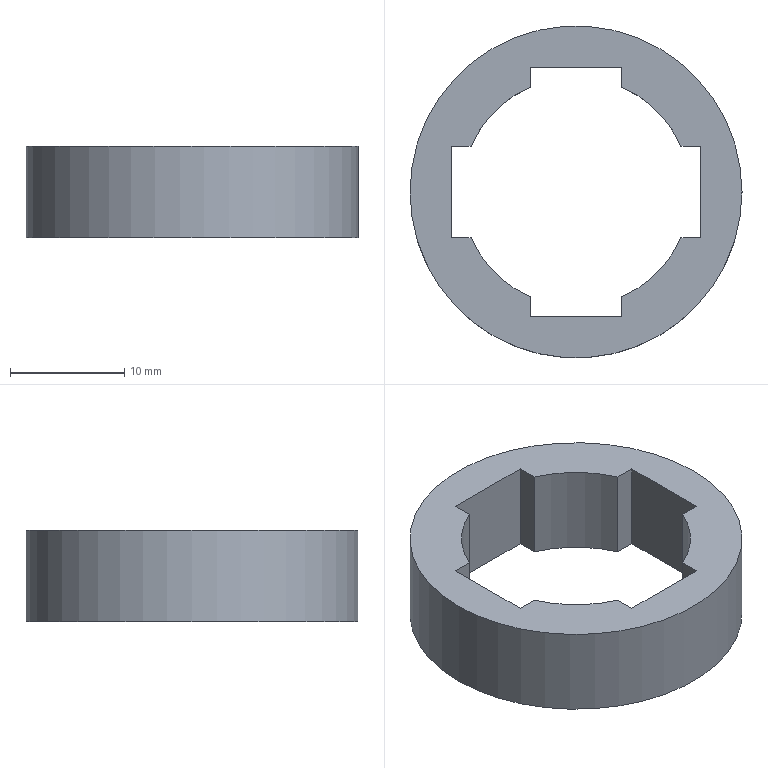Part | NX | features DATUM_CSYS 2, EXTRUDE 1, SKETCH 1 | 1 solid | 19 faces | box 29 x 29 x 8 mm | volume 2471 mm3 | plane 14 | cylinder 5 | commonest cylinder face diameters 20 x4 29 x1
STEP:
#1=CARTESIAN_POINT('',(-10.9,-4.,0.));
#2=VERTEX_POINT('',#1);
#3=CARTESIAN_POINT('',(-10.9,4.,0.));
#4=VERTEX_POINT('',#3);
#5=CARTESIAN_POINT('',(-10.9,2.1,0.));
#6=DIRECTION('',(0.,1.,0.));
#7=VECTOR('',#6,1000.);
#8=LINE('',#5,#7);
#9=EDGE_CURVE('',#2,#4,#8,.T.);
#10=ORIENTED_EDGE('',*,*,#9,.T.);
#11=CARTESIAN_POINT('',(-10.9,4.,8.));
#12=VERTEX_POINT('',#11);
#13=CARTESIAN_POINT('',(-10.9,4.,8.));
#14=DIRECTION('',(0.,0.,-1.));
#15=VECTOR('',#14,1000.);
#16=LINE('',#13,#15);
#17=EDGE_CURVE('',#12,#4,#16,.T.);
#18=ORIENTED_EDGE('',*,*,#17,.F.);
#19=CARTESIAN_POINT('',(-10.9,-4.,8.));
#20=VERTEX_POINT('',#19);
#21=CARTESIAN_POINT('',(-10.9,-4.,8.));
#22=DIRECTION('',(0.,1.,0.));
#23=VECTOR('',#22,1000.);
#24=LINE('',#21,#23);
#25=EDGE_CURVE('',#20,#12,#24,.T.);
#26=ORIENTED_EDGE('',*,*,#25,.F.);
#27=CARTESIAN_POINT('',(-10.9,-4.,8.));
#28=DIRECTION('',(0.,0.,-1.));
#29=VECTOR('',#28,1000.);
#30=LINE('',#27,#29);
#31=EDGE_CURVE('',#20,#2,#30,.T.);
#32=ORIENTED_EDGE('',*,*,#31,.T.);
#33=EDGE_LOOP('',(#10,#18,#26,#32));
#34=FACE_BOUND('',#33,.T.);
#35=CARTESIAN_POINT('',(-10.9,2.1,8.));
#36=DIRECTION('',(-1.,0.,0.));
#37=DIRECTION('',(0.,0.,1.));
#38=AXIS2_PLACEMENT_3D('',#35,#36,#37);
#39=PLANE('',#38);
#40=ADVANCED_FACE('',(#34),#39,.F.);
#41=CARTESIAN_POINT('',(-9.165,4.,0.));
#42=VERTEX_POINT('',#41);
#43=CARTESIAN_POINT('',(-10.9,4.,0.));
#44=DIRECTION('',(1.,0.,0.));
#45=VECTOR('',#44,1000.);
#46=LINE('',#43,#45);
#47=EDGE_CURVE('',#4,#42,#46,.T.);
#48=ORIENTED_EDGE('',*,*,#47,.T.);
#49=CARTESIAN_POINT('',(-9.165,4.,8.));
#50=VERTEX_POINT('',#49);
#51=CARTESIAN_POINT('',(-9.165,4.,8.));
#52=DIRECTION('',(0.,0.,-1.));
#53=VECTOR('',#52,1000.);
#54=LINE('',#51,#53);
#55=EDGE_CURVE('',#50,#42,#54,.T.);
#56=ORIENTED_EDGE('',*,*,#55,.F.);
#57=CARTESIAN_POINT('',(-10.9,4.,8.));
#58=DIRECTION('',(1.,0.,0.));
#59=VECTOR('',#58,1000.);
#60=LINE('',#57,#59);
#61=EDGE_CURVE('',#12,#50,#60,.T.);
#62=ORIENTED_EDGE('',*,*,#61,.F.);
#63=ORIENTED_EDGE('',*,*,#17,.T.);
#64=EDGE_LOOP('',(#48,#56,#62,#63));
#65=FACE_BOUND('',#64,.T.);
#66=CARTESIAN_POINT('',(-10.9,4.,8.));
#67=DIRECTION('',(0.,1.,0.));
#68=DIRECTION('',(0.,0.,1.));
#69=AXIS2_PLACEMENT_3D('',#66,#67,#68);
#70=PLANE('',#69);
#71=ADVANCED_FACE('',(#65),#70,.F.);
#72=CARTESIAN_POINT('',(-4.,9.165,0.));
#73=VERTEX_POINT('',#72);
#74=CARTESIAN_POINT('',(0.,0.,0.));
#75=DIRECTION('',(0.,0.,-1.));
#76=DIRECTION('',(1.,0.,0.));
#77=AXIS2_PLACEMENT_3D('',#74,#75,#76);
#78=CIRCLE('',#77,10.);
#79=EDGE_CURVE('',#42,#73,#78,.T.);
#80=ORIENTED_EDGE('',*,*,#79,.T.);
#81=CARTESIAN_POINT('',(-4.,9.165,8.));
#82=VERTEX_POINT('',#81);
#83=CARTESIAN_POINT('',(-4.,9.165,8.));
#84=DIRECTION('',(0.,0.,-1.));
#85=VECTOR('',#84,1000.);
#86=LINE('',#83,#85);
#87=EDGE_CURVE('',#82,#73,#86,.T.);
#88=ORIENTED_EDGE('',*,*,#87,.F.);
#89=CARTESIAN_POINT('',(0.,0.,8.));
#90=DIRECTION('',(0.,0.,-1.));
#91=DIRECTION('',(1.,0.,0.));
#92=AXIS2_PLACEMENT_3D('',#89,#90,#91);
#93=CIRCLE('',#92,10.);
#94=EDGE_CURVE('',#50,#82,#93,.T.);
#95=ORIENTED_EDGE('',*,*,#94,.F.);
#96=ORIENTED_EDGE('',*,*,#55,.T.);
#97=EDGE_LOOP('',(#80,#88,#95,#96));
#98=FACE_BOUND('',#97,.T.);
#99=CARTESIAN_POINT('',(0.,0.,8.));
#100=DIRECTION('',(0.,0.,-1.));
#101=DIRECTION('',(-1.,0.,0.));
#102=AXIS2_PLACEMENT_3D('',#99,#100,#101);
#103=CYLINDRICAL_SURFACE('',#102,10.);
#104=ADVANCED_FACE('',(#98),#103,.F.);
#105=CARTESIAN_POINT('',(-4.,10.9,0.));
#106=VERTEX_POINT('',#105);
#107=CARTESIAN_POINT('',(-4.,9.165,0.));
#108=DIRECTION('',(0.,1.,0.));
#109=VECTOR('',#108,1000.);
#110=LINE('',#107,#109);
#111=EDGE_CURVE('',#73,#106,#110,.T.);
#112=ORIENTED_EDGE('',*,*,#111,.T.);
#113=CARTESIAN_POINT('',(-4.,10.9,8.));
#114=VERTEX_POINT('',#113);
#115=CARTESIAN_POINT('',(-4.,10.9,8.));
#116=DIRECTION('',(0.,0.,-1.));
#117=VECTOR('',#116,1000.);
#118=LINE('',#115,#117);
#119=EDGE_CURVE('',#114,#106,#118,.T.);
#120=ORIENTED_EDGE('',*,*,#119,.F.);
#121=CARTESIAN_POINT('',(-4.,9.165,8.));
#122=DIRECTION('',(0.,1.,0.));
#123=VECTOR('',#122,1000.);
#124=LINE('',#121,#123);
#125=EDGE_CURVE('',#82,#114,#124,.T.);
#126=ORIENTED_EDGE('',*,*,#125,.F.);
#127=ORIENTED_EDGE('',*,*,#87,.T.);
#128=EDGE_LOOP('',(#112,#120,#126,#127));
#129=FACE_BOUND('',#128,.T.);
#130=CARTESIAN_POINT('',(-4.,9.165,8.));
#131=DIRECTION('',(-1.,0.,0.));
#132=DIRECTION('',(0.,0.,1.));
#133=AXIS2_PLACEMENT_3D('',#130,#131,#132);
#134=PLANE('',#133);
#135=ADVANCED_FACE('',(#129),#134,.F.);
#136=CARTESIAN_POINT('',(4.,10.9,0.));
#137=VERTEX_POINT('',#136);
#138=CARTESIAN_POINT('',(-2.1,10.9,0.));
#139=DIRECTION('',(1.,0.,0.));
#140=VECTOR('',#139,1000.);
#141=LINE('',#138,#140);
#142=EDGE_CURVE('',#106,#137,#141,.T.);
#143=ORIENTED_EDGE('',*,*,#142,.T.);
#144=CARTESIAN_POINT('',(4.,10.9,8.));
#145=VERTEX_POINT('',#144);
#146=CARTESIAN_POINT('',(4.,10.9,8.));
#147=DIRECTION('',(0.,0.,-1.));
#148=VECTOR('',#147,1000.);
#149=LINE('',#146,#148);
#150=EDGE_CURVE('',#145,#137,#149,.T.);
#151=ORIENTED_EDGE('',*,*,#150,.F.);
#152=CARTESIAN_POINT('',(-4.,10.9,8.));
#153=DIRECTION('',(1.,0.,0.));
#154=VECTOR('',#153,1000.);
#155=LINE('',#152,#154);
#156=EDGE_CURVE('',#114,#145,#155,.T.);
#157=ORIENTED_EDGE('',*,*,#156,.F.);
#158=ORIENTED_EDGE('',*,*,#119,.T.);
#159=EDGE_LOOP('',(#143,#151,#157,#158));
#160=FACE_BOUND('',#159,.T.);
#161=CARTESIAN_POINT('',(-2.1,10.9,8.));
#162=DIRECTION('',(0.,1.,0.));
#163=DIRECTION('',(0.,0.,1.));
#164=AXIS2_PLACEMENT_3D('',#161,#162,#163);
#165=PLANE('',#164);
#166=ADVANCED_FACE('',(#160),#165,.F.);
#167=CARTESIAN_POINT('',(4.,9.165,0.));
#168=VERTEX_POINT('',#167);
#169=CARTESIAN_POINT('',(4.,10.9,0.));
#170=DIRECTION('',(0.,-1.,0.));
#171=VECTOR('',#170,1000.);
#172=LINE('',#169,#171);
#173=EDGE_CURVE('',#137,#168,#172,.T.);
#174=ORIENTED_EDGE('',*,*,#173,.T.);
#175=CARTESIAN_POINT('',(4.,9.165,8.));
#176=VERTEX_POINT('',#175);
#177=CARTESIAN_POINT('',(4.,9.165,8.));
#178=DIRECTION('',(0.,0.,-1.));
#179=VECTOR('',#178,1000.);
#180=LINE('',#177,#179);
#181=EDGE_CURVE('',#176,#168,#180,.T.);
#182=ORIENTED_EDGE('',*,*,#181,.F.);
#183=CARTESIAN_POINT('',(4.,10.9,8.));
#184=DIRECTION('',(0.,-1.,0.));
#185=VECTOR('',#184,1000.);
#186=LINE('',#183,#185);
#187=EDGE_CURVE('',#145,#176,#186,.T.);
#188=ORIENTED_EDGE('',*,*,#187,.F.);
#189=ORIENTED_EDGE('',*,*,#150,.T.);
#190=EDGE_LOOP('',(#174,#182,#188,#189));
#191=FACE_BOUND('',#190,.T.);
#192=CARTESIAN_POINT('',(4.,10.9,8.));
#193=DIRECTION('',(1.,0.,0.));
#194=DIRECTION('',(0.,0.,-1.));
#195=AXIS2_PLACEMENT_3D('',#192,#193,#194);
#196=PLANE('',#195);
#197=ADVANCED_FACE('',(#191),#196,.F.);
#198=CARTESIAN_POINT('',(9.165,4.,0.));
#199=VERTEX_POINT('',#198);
#200=CARTESIAN_POINT('',(0.,0.,0.));
#201=DIRECTION('',(0.,0.,-1.));
#202=DIRECTION('',(1.,0.,0.));
#203=AXIS2_PLACEMENT_3D('',#200,#201,#202);
#204=CIRCLE('',#203,10.);
#205=EDGE_CURVE('',#168,#199,#204,.T.);
#206=ORIENTED_EDGE('',*,*,#205,.T.);
#207=CARTESIAN_POINT('',(9.165,4.,8.));
#208=VERTEX_POINT('',#207);
#209=CARTESIAN_POINT('',(9.165,4.,8.));
#210=DIRECTION('',(0.,0.,-1.));
#211=VECTOR('',#210,1000.);
#212=LINE('',#209,#211);
#213=EDGE_CURVE('',#208,#199,#212,.T.);
#214=ORIENTED_EDGE('',*,*,#213,.F.);
#215=CARTESIAN_POINT('',(0.,0.,8.));
#216=DIRECTION('',(0.,0.,-1.));
#217=DIRECTION('',(1.,0.,0.));
#218=AXIS2_PLACEMENT_3D('',#215,#216,#217);
#219=CIRCLE('',#218,10.);
#220=EDGE_CURVE('',#176,#208,#219,.T.);
#221=ORIENTED_EDGE('',*,*,#220,.F.);
#222=ORIENTED_EDGE('',*,*,#181,.T.);
#223=EDGE_LOOP('',(#206,#214,#221,#222));
#224=FACE_BOUND('',#223,.T.);
#225=CARTESIAN_POINT('',(0.,0.,8.));
#226=DIRECTION('',(0.,0.,-1.));
#227=DIRECTION('',(-1.,0.,0.));
#228=AXIS2_PLACEMENT_3D('',#225,#226,#227);
#229=CYLINDRICAL_SURFACE('',#228,10.);
#230=ADVANCED_FACE('',(#224),#229,.F.);
#231=CARTESIAN_POINT('',(10.9,4.,0.));
#232=VERTEX_POINT('',#231);
#233=CARTESIAN_POINT('',(9.165,4.,0.));
#234=DIRECTION('',(1.,0.,0.));
#235=VECTOR('',#234,1000.);
#236=LINE('',#233,#235);
#237=EDGE_CURVE('',#199,#232,#236,.T.);
#238=ORIENTED_EDGE('',*,*,#237,.T.);
#239=CARTESIAN_POINT('',(10.9,4.,8.));
#240=VERTEX_POINT('',#239);
#241=CARTESIAN_POINT('',(10.9,4.,8.));
#242=DIRECTION('',(0.,0.,-1.));
#243=VECTOR('',#242,1000.);
#244=LINE('',#241,#243);
#245=EDGE_CURVE('',#240,#232,#244,.T.);
#246=ORIENTED_EDGE('',*,*,#245,.F.);
#247=CARTESIAN_POINT('',(9.165,4.,8.));
#248=DIRECTION('',(1.,0.,0.));
#249=VECTOR('',#248,1000.);
#250=LINE('',#247,#249);
#251=EDGE_CURVE('',#208,#240,#250,.T.);
#252=ORIENTED_EDGE('',*,*,#251,.F.);
#253=ORIENTED_EDGE('',*,*,#213,.T.);
#254=EDGE_LOOP('',(#238,#246,#252,#253));
#255=FACE_BOUND('',#254,.T.);
#256=CARTESIAN_POINT('',(9.165,4.,8.));
#257=DIRECTION('',(0.,1.,0.));
#258=DIRECTION('',(0.,0.,1.));
#259=AXIS2_PLACEMENT_3D('',#256,#257,#258);
#260=PLANE('',#259);
#261=ADVANCED_FACE('',(#255),#260,.F.);
#262=CARTESIAN_POINT('',(10.9,-4.,0.));
#263=VERTEX_POINT('',#262);
#264=CARTESIAN_POINT('',(10.9,-2.1,0.));
#265=DIRECTION('',(0.,-1.,0.));
#266=VECTOR('',#265,1000.);
#267=LINE('',#264,#266);
#268=EDGE_CURVE('',#232,#263,#267,.T.);
#269=ORIENTED_EDGE('',*,*,#268,.T.);
#270=CARTESIAN_POINT('',(10.9,-4.,8.));
#271=VERTEX_POINT('',#270);
#272=CARTESIAN_POINT('',(10.9,-4.,8.));
#273=DIRECTION('',(0.,0.,-1.));
#274=VECTOR('',#273,1000.);
#275=LINE('',#272,#274);
#276=EDGE_CURVE('',#271,#263,#275,.T.);
#277=ORIENTED_EDGE('',*,*,#276,.F.);
#278=CARTESIAN_POINT('',(10.9,4.,8.));
#279=DIRECTION('',(0.,-1.,0.));
#280=VECTOR('',#279,1000.);
#281=LINE('',#278,#280);
#282=EDGE_CURVE('',#240,#271,#281,.T.);
#283=ORIENTED_EDGE('',*,*,#282,.F.);
#284=ORIENTED_EDGE('',*,*,#245,.T.);
#285=EDGE_LOOP('',(#269,#277,#283,#284));
#286=FACE_BOUND('',#285,.T.);
#287=CARTESIAN_POINT('',(10.9,-2.1,8.));
#288=DIRECTION('',(1.,0.,0.));
#289=DIRECTION('',(0.,0.,-1.));
#290=AXIS2_PLACEMENT_3D('',#287,#288,#289);
#291=PLANE('',#290);
#292=ADVANCED_FACE('',(#286),#291,.F.);
#293=CARTESIAN_POINT('',(9.165,-4.,0.));
#294=VERTEX_POINT('',#293);
#295=CARTESIAN_POINT('',(10.9,-4.,0.));
#296=DIRECTION('',(-1.,0.,0.));
#297=VECTOR('',#296,1000.);
#298=LINE('',#295,#297);
#299=EDGE_CURVE('',#263,#294,#298,.T.);
#300=ORIENTED_EDGE('',*,*,#299,.T.);
#301=CARTESIAN_POINT('',(9.165,-4.,8.));
#302=VERTEX_POINT('',#301);
#303=CARTESIAN_POINT('',(9.165,-4.,8.));
#304=DIRECTION('',(0.,0.,-1.));
#305=VECTOR('',#304,1000.);
#306=LINE('',#303,#305);
#307=EDGE_CURVE('',#302,#294,#306,.T.);
#308=ORIENTED_EDGE('',*,*,#307,.F.);
#309=CARTESIAN_POINT('',(10.9,-4.,8.));
#310=DIRECTION('',(-1.,0.,0.));
#311=VECTOR('',#310,1000.);
#312=LINE('',#309,#311);
#313=EDGE_CURVE('',#271,#302,#312,.T.);
#314=ORIENTED_EDGE('',*,*,#313,.F.);
#315=ORIENTED_EDGE('',*,*,#276,.T.);
#316=EDGE_LOOP('',(#300,#308,#314,#315));
#317=FACE_BOUND('',#316,.T.);
#318=CARTESIAN_POINT('',(10.9,-4.,8.));
#319=DIRECTION('',(0.,-1.,0.));
#320=DIRECTION('',(0.,0.,-1.));
#321=AXIS2_PLACEMENT_3D('',#318,#319,#320);
#322=PLANE('',#321);
#323=ADVANCED_FACE('',(#317),#322,.F.);
#324=CARTESIAN_POINT('',(4.,-9.165,0.));
#325=VERTEX_POINT('',#324);
#326=CARTESIAN_POINT('',(0.,0.,0.));
#327=DIRECTION('',(0.,0.,-1.));
#328=DIRECTION('',(1.,0.,0.));
#329=AXIS2_PLACEMENT_3D('',#326,#327,#328);
#330=CIRCLE('',#329,10.);
#331=EDGE_CURVE('',#294,#325,#330,.T.);
#332=ORIENTED_EDGE('',*,*,#331,.T.);
#333=CARTESIAN_POINT('',(4.,-9.165,8.));
#334=VERTEX_POINT('',#333);
#335=CARTESIAN_POINT('',(4.,-9.165,8.));
#336=DIRECTION('',(0.,0.,-1.));
#337=VECTOR('',#336,1000.);
#338=LINE('',#335,#337);
#339=EDGE_CURVE('',#334,#325,#338,.T.);
#340=ORIENTED_EDGE('',*,*,#339,.F.);
#341=CARTESIAN_POINT('',(0.,0.,8.));
#342=DIRECTION('',(0.,0.,-1.));
#343=DIRECTION('',(1.,0.,0.));
#344=AXIS2_PLACEMENT_3D('',#341,#342,#343);
#345=CIRCLE('',#344,10.);
#346=EDGE_CURVE('',#302,#334,#345,.T.);
#347=ORIENTED_EDGE('',*,*,#346,.F.);
#348=ORIENTED_EDGE('',*,*,#307,.T.);
#349=EDGE_LOOP('',(#332,#340,#347,#348));
#350=FACE_BOUND('',#349,.T.);
#351=CARTESIAN_POINT('',(0.,0.,8.));
#352=DIRECTION('',(0.,0.,-1.));
#353=DIRECTION('',(-1.,0.,0.));
#354=AXIS2_PLACEMENT_3D('',#351,#352,#353);
#355=CYLINDRICAL_SURFACE('',#354,10.);
#356=ADVANCED_FACE('',(#350),#355,.F.);
#357=CARTESIAN_POINT('',(4.,-10.9,0.));
#358=VERTEX_POINT('',#357);
#359=CARTESIAN_POINT('',(4.,-9.165,0.));
#360=DIRECTION('',(0.,-1.,0.));
#361=VECTOR('',#360,1000.);
#362=LINE('',#359,#361);
#363=EDGE_CURVE('',#325,#358,#362,.T.);
#364=ORIENTED_EDGE('',*,*,#363,.T.);
#365=CARTESIAN_POINT('',(4.,-10.9,8.));
#366=VERTEX_POINT('',#365);
#367=CARTESIAN_POINT('',(4.,-10.9,8.));
#368=DIRECTION('',(0.,0.,-1.));
#369=VECTOR('',#368,1000.);
#370=LINE('',#367,#369);
#371=EDGE_CURVE('',#366,#358,#370,.T.);
#372=ORIENTED_EDGE('',*,*,#371,.F.);
#373=CARTESIAN_POINT('',(4.,-9.165,8.));
#374=DIRECTION('',(0.,-1.,0.));
#375=VECTOR('',#374,1000.);
#376=LINE('',#373,#375);
#377=EDGE_CURVE('',#334,#366,#376,.T.);
#378=ORIENTED_EDGE('',*,*,#377,.F.);
#379=ORIENTED_EDGE('',*,*,#339,.T.);
#380=EDGE_LOOP('',(#364,#372,#378,#379));
#381=FACE_BOUND('',#380,.T.);
#382=CARTESIAN_POINT('',(4.,-9.165,8.));
#383=DIRECTION('',(1.,0.,0.));
#384=DIRECTION('',(0.,0.,-1.));
#385=AXIS2_PLACEMENT_3D('',#382,#383,#384);
#386=PLANE('',#385);
#387=ADVANCED_FACE('',(#381),#386,.F.);
#388=CARTESIAN_POINT('',(-4.,-10.9,0.));
#389=VERTEX_POINT('',#388);
#390=CARTESIAN_POINT('',(-2.1,-10.9,0.));
#391=DIRECTION('',(-1.,0.,0.));
#392=VECTOR('',#391,1000.);
#393=LINE('',#390,#392);
#394=EDGE_CURVE('',#358,#389,#393,.T.);
#395=ORIENTED_EDGE('',*,*,#394,.T.);
#396=CARTESIAN_POINT('',(-4.,-10.9,8.));
#397=VERTEX_POINT('',#396);
#398=CARTESIAN_POINT('',(-4.,-10.9,8.));
#399=DIRECTION('',(0.,0.,-1.));
#400=VECTOR('',#399,1000.);
#401=LINE('',#398,#400);
#402=EDGE_CURVE('',#397,#389,#401,.T.);
#403=ORIENTED_EDGE('',*,*,#402,.F.);
#404=CARTESIAN_POINT('',(4.,-10.9,8.));
#405=DIRECTION('',(-1.,0.,0.));
#406=VECTOR('',#405,1000.);
#407=LINE('',#404,#406);
#408=EDGE_CURVE('',#366,#397,#407,.T.);
#409=ORIENTED_EDGE('',*,*,#408,.F.);
#410=ORIENTED_EDGE('',*,*,#371,.T.);
#411=EDGE_LOOP('',(#395,#403,#409,#410));
#412=FACE_BOUND('',#411,.T.);
#413=CARTESIAN_POINT('',(-2.1,-10.9,8.));
#414=DIRECTION('',(0.,-1.,0.));
#415=DIRECTION('',(0.,0.,-1.));
#416=AXIS2_PLACEMENT_3D('',#413,#414,#415);
#417=PLANE('',#416);
#418=ADVANCED_FACE('',(#412),#417,.F.);
#419=CARTESIAN_POINT('',(-4.,-9.165,0.));
#420=VERTEX_POINT('',#419);
#421=CARTESIAN_POINT('',(-4.,-10.9,0.));
#422=DIRECTION('',(0.,1.,0.));
#423=VECTOR('',#422,1000.);
#424=LINE('',#421,#423);
#425=EDGE_CURVE('',#389,#420,#424,.T.);
#426=ORIENTED_EDGE('',*,*,#425,.T.);
#427=CARTESIAN_POINT('',(-4.,-9.165,8.));
#428=VERTEX_POINT('',#427);
#429=CARTESIAN_POINT('',(-4.,-9.165,8.));
#430=DIRECTION('',(0.,0.,-1.));
#431=VECTOR('',#430,1000.);
#432=LINE('',#429,#431);
#433=EDGE_CURVE('',#428,#420,#432,.T.);
#434=ORIENTED_EDGE('',*,*,#433,.F.);
#435=CARTESIAN_POINT('',(-4.,-10.9,8.));
#436=DIRECTION('',(0.,1.,0.));
#437=VECTOR('',#436,1000.);
#438=LINE('',#435,#437);
#439=EDGE_CURVE('',#397,#428,#438,.T.);
#440=ORIENTED_EDGE('',*,*,#439,.F.);
#441=ORIENTED_EDGE('',*,*,#402,.T.);
#442=EDGE_LOOP('',(#426,#434,#440,#441));
#443=FACE_BOUND('',#442,.T.);
#444=CARTESIAN_POINT('',(-4.,-10.9,8.));
#445=DIRECTION('',(-1.,0.,0.));
#446=DIRECTION('',(0.,0.,1.));
#447=AXIS2_PLACEMENT_3D('',#444,#445,#446);
#448=PLANE('',#447);
#449=ADVANCED_FACE('',(#443),#448,.F.);
#450=CARTESIAN_POINT('',(-9.165,-4.,0.));
#451=VERTEX_POINT('',#450);
#452=CARTESIAN_POINT('',(0.,0.,0.));
#453=DIRECTION('',(0.,0.,-1.));
#454=DIRECTION('',(1.,0.,0.));
#455=AXIS2_PLACEMENT_3D('',#452,#453,#454);
#456=CIRCLE('',#455,10.);
#457=EDGE_CURVE('',#420,#451,#456,.T.);
#458=ORIENTED_EDGE('',*,*,#457,.T.);
#459=CARTESIAN_POINT('',(-9.165,-4.,8.));
#460=VERTEX_POINT('',#459);
#461=CARTESIAN_POINT('',(-9.165,-4.,8.));
#462=DIRECTION('',(0.,0.,-1.));
#463=VECTOR('',#462,1000.);
#464=LINE('',#461,#463);
#465=EDGE_CURVE('',#460,#451,#464,.T.);
#466=ORIENTED_EDGE('',*,*,#465,.F.);
#467=CARTESIAN_POINT('',(0.,0.,8.));
#468=DIRECTION('',(0.,0.,-1.));
#469=DIRECTION('',(1.,0.,0.));
#470=AXIS2_PLACEMENT_3D('',#467,#468,#469);
#471=CIRCLE('',#470,10.);
#472=EDGE_CURVE('',#428,#460,#471,.T.);
#473=ORIENTED_EDGE('',*,*,#472,.F.);
#474=ORIENTED_EDGE('',*,*,#433,.T.);
#475=EDGE_LOOP('',(#458,#466,#473,#474));
#476=FACE_BOUND('',#475,.T.);
#477=CARTESIAN_POINT('',(0.,0.,8.));
#478=DIRECTION('',(0.,0.,-1.));
#479=DIRECTION('',(-1.,0.,0.));
#480=AXIS2_PLACEMENT_3D('',#477,#478,#479);
#481=CYLINDRICAL_SURFACE('',#480,10.);
#482=ADVANCED_FACE('',(#476),#481,.F.);
#483=CARTESIAN_POINT('',(14.5,0.,8.));
#484=VERTEX_POINT('',#483);
#485=CARTESIAN_POINT('',(0.,0.,8.));
#486=DIRECTION('',(0.,0.,1.));
#487=DIRECTION('',(1.,0.,0.));
#488=AXIS2_PLACEMENT_3D('',#485,#486,#487);
#489=CIRCLE('',#488,14.5);
#490=EDGE_CURVE('',#484,#484,#489,.T.);
#491=ORIENTED_EDGE('',*,*,#490,.F.);
#492=EDGE_LOOP('',(#491));
#493=FACE_BOUND('',#492,.T.);
#494=CARTESIAN_POINT('',(14.5,0.,0.));
#495=VERTEX_POINT('',#494);
#496=CARTESIAN_POINT('',(0.,0.,0.));
#497=DIRECTION('',(0.,0.,1.));
#498=DIRECTION('',(1.,0.,0.));
#499=AXIS2_PLACEMENT_3D('',#496,#497,#498);
#500=CIRCLE('',#499,14.5);
#501=EDGE_CURVE('',#495,#495,#500,.T.);
#502=ORIENTED_EDGE('',*,*,#501,.T.);
#503=EDGE_LOOP('',(#502));
#504=FACE_BOUND('',#503,.T.);
#505=CARTESIAN_POINT('',(0.,0.,8.));
#506=DIRECTION('',(0.,0.,-1.));
#507=DIRECTION('',(-1.,0.,0.));
#508=AXIS2_PLACEMENT_3D('',#505,#506,#507);
#509=CYLINDRICAL_SURFACE('',#508,14.5);
#510=ADVANCED_FACE('',(#493,#504),#509,.T.);
#511=CARTESIAN_POINT('',(-9.165,-4.,0.));
#512=DIRECTION('',(-1.,0.,0.));
#513=VECTOR('',#512,1000.);
#514=LINE('',#511,#513);
#515=EDGE_CURVE('',#451,#2,#514,.T.);
#516=ORIENTED_EDGE('',*,*,#515,.T.);
#517=ORIENTED_EDGE('',*,*,#31,.F.);
#518=CARTESIAN_POINT('',(-9.165,-4.,8.));
#519=DIRECTION('',(-1.,0.,0.));
#520=VECTOR('',#519,1000.);
#521=LINE('',#518,#520);
#522=EDGE_CURVE('',#460,#20,#521,.T.);
#523=ORIENTED_EDGE('',*,*,#522,.F.);
#524=ORIENTED_EDGE('',*,*,#465,.T.);
#525=EDGE_LOOP('',(#516,#517,#523,#524));
#526=FACE_BOUND('',#525,.T.);
#527=CARTESIAN_POINT('',(-9.165,-4.,8.));
#528=DIRECTION('',(0.,-1.,0.));
#529=DIRECTION('',(0.,0.,-1.));
#530=AXIS2_PLACEMENT_3D('',#527,#528,#529);
#531=PLANE('',#530);
#532=ADVANCED_FACE('',(#526),#531,.F.);
#533=ORIENTED_EDGE('',*,*,#490,.T.);
#534=EDGE_LOOP('',(#533));
#535=FACE_BOUND('',#534,.T.);
#536=ORIENTED_EDGE('',*,*,#25,.T.);
#537=ORIENTED_EDGE('',*,*,#61,.T.);
#538=ORIENTED_EDGE('',*,*,#94,.T.);
#539=ORIENTED_EDGE('',*,*,#125,.T.);
#540=ORIENTED_EDGE('',*,*,#156,.T.);
#541=ORIENTED_EDGE('',*,*,#187,.T.);
#542=ORIENTED_EDGE('',*,*,#220,.T.);
#543=ORIENTED_EDGE('',*,*,#251,.T.);
#544=ORIENTED_EDGE('',*,*,#282,.T.);
#545=ORIENTED_EDGE('',*,*,#313,.T.);
#546=ORIENTED_EDGE('',*,*,#346,.T.);
#547=ORIENTED_EDGE('',*,*,#377,.T.);
#548=ORIENTED_EDGE('',*,*,#408,.T.);
#549=ORIENTED_EDGE('',*,*,#439,.T.);
#550=ORIENTED_EDGE('',*,*,#472,.T.);
#551=ORIENTED_EDGE('',*,*,#522,.T.);
#552=EDGE_LOOP('',(#536,#537,#538,#539,#540,#541,#542,#543,#544,#545,#546,#547,#548,#549,#550,#551));
#553=FACE_BOUND('',#552,.T.);
#554=CARTESIAN_POINT('',(0.,0.,8.));
#555=DIRECTION('',(0.,0.,1.));
#556=DIRECTION('',(1.,0.,0.));
#557=AXIS2_PLACEMENT_3D('',#554,#555,#556);
#558=PLANE('',#557);
#559=ADVANCED_FACE('',(#535,#553),#558,.T.);
#560=ORIENTED_EDGE('',*,*,#501,.F.);
#561=EDGE_LOOP('',(#560));
#562=FACE_BOUND('',#561,.T.);
#563=ORIENTED_EDGE('',*,*,#9,.F.);
#564=ORIENTED_EDGE('',*,*,#515,.F.);
#565=ORIENTED_EDGE('',*,*,#457,.F.);
#566=ORIENTED_EDGE('',*,*,#425,.F.);
#567=ORIENTED_EDGE('',*,*,#394,.F.);
#568=ORIENTED_EDGE('',*,*,#363,.F.);
#569=ORIENTED_EDGE('',*,*,#331,.F.);
#570=ORIENTED_EDGE('',*,*,#299,.F.);
#571=ORIENTED_EDGE('',*,*,#268,.F.);
#572=ORIENTED_EDGE('',*,*,#237,.F.);
#573=ORIENTED_EDGE('',*,*,#205,.F.);
#574=ORIENTED_EDGE('',*,*,#173,.F.);
#575=ORIENTED_EDGE('',*,*,#142,.F.);
#576=ORIENTED_EDGE('',*,*,#111,.F.);
#577=ORIENTED_EDGE('',*,*,#79,.F.);
#578=ORIENTED_EDGE('',*,*,#47,.F.);
#579=EDGE_LOOP('',(#563,#564,#565,#566,#567,#568,#569,#570,#571,#572,#573,#574,#575,#576,#577,#578));
#580=FACE_BOUND('',#579,.T.);
#581=CARTESIAN_POINT('',(0.,0.,0.));
#582=DIRECTION('',(0.,0.,1.));
#583=DIRECTION('',(1.,0.,0.));
#584=AXIS2_PLACEMENT_3D('',#581,#582,#583);
#585=PLANE('',#584);
#586=ADVANCED_FACE('',(#562,#580),#585,.F.);
#587=CLOSED_SHELL('',(#40,#71,#104,#135,#166,#197,#230,#261,#292,#323,#356,#387,#418,#449,#482,#510,#532,#559,#586));
#588=MANIFOLD_SOLID_BREP('',#587);
#589=(LENGTH_UNIT()NAMED_UNIT(*)SI_UNIT(.MILLI.,.METRE.));
#590=UNCERTAINTY_MEASURE_WITH_UNIT(LENGTH_MEASURE(0.00001),#589,'','');
#591=(NAMED_UNIT(*)PLANE_ANGLE_UNIT()SI_UNIT($,.RADIAN.));
#592=(NAMED_UNIT(*)SI_UNIT($,.STERADIAN.)SOLID_ANGLE_UNIT());
#593=(GEOMETRIC_REPRESENTATION_CONTEXT(3)GLOBAL_UNCERTAINTY_ASSIGNED_CONTEXT((#590))GLOBAL_UNIT_ASSIGNED_CONTEXT((#589,#591,#592))REPRESENTATION_CONTEXT('',''));
#594=ADVANCED_BREP_SHAPE_REPRESENTATION('',(#588),#593);